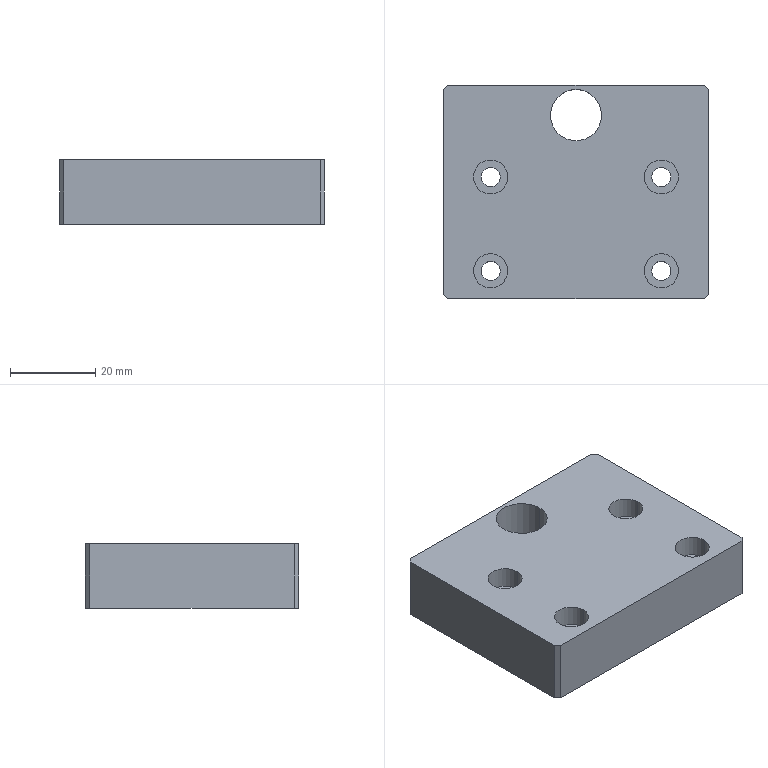Part | STEP file | 227H056245 Move Block_Default | 1 solid | 32 faces | box 62 x 50 x 15 mm | volume 43132 mm3 | cylinder 18 | plane 14 | commonest cylinder face diameters 4.5 x8 8 x8 12 x2